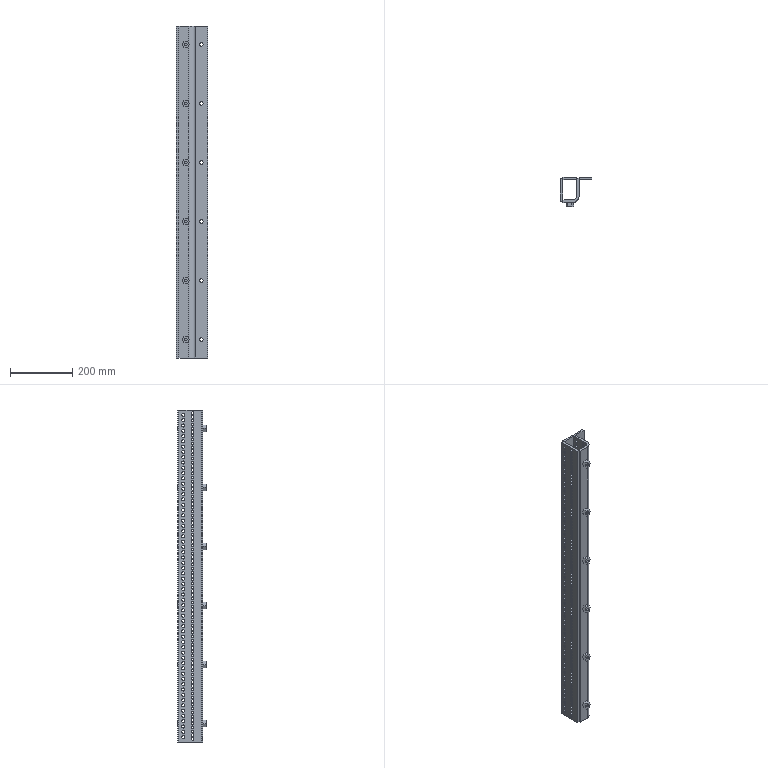Part | STEP file | Positioning slot assembly 1_Default<As machined> | 10 solids | 708 faces | box 100 x 92 x 1069 mm | volume 2012408 mm3 | cylinder 634 | plane 74 | commonest cylinder face diameters 8 x348 10 x248 8.5 x12 11 x12 14 x12 24 x1